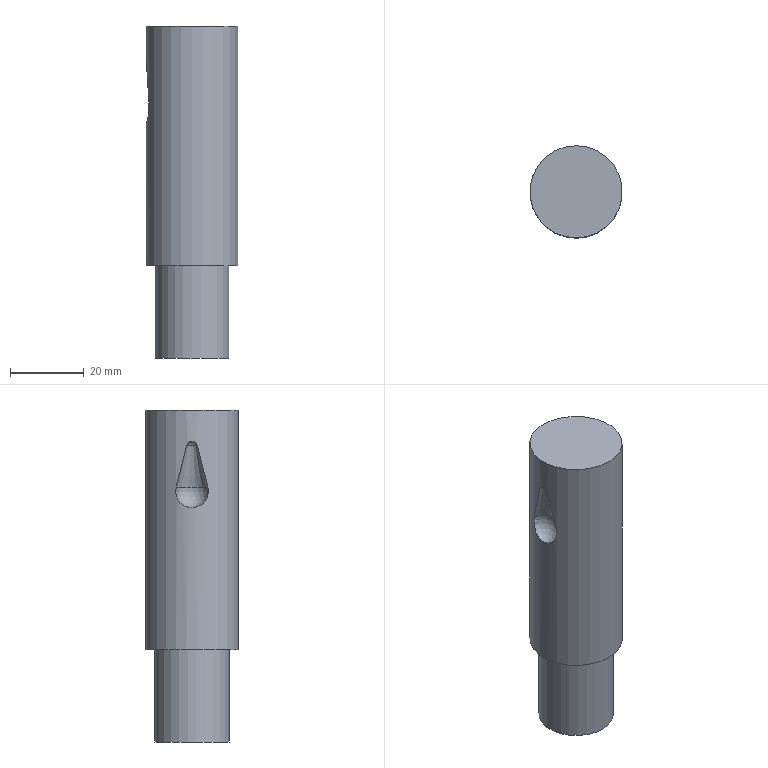Part | NX | features solid 2 | 1 solid | 8 faces | volume 39563 mm3 | plane 3 | cylinder 2 | sphere 2 | cone 1 | commonest cylinder face diameters 20.1 x1 25 x1